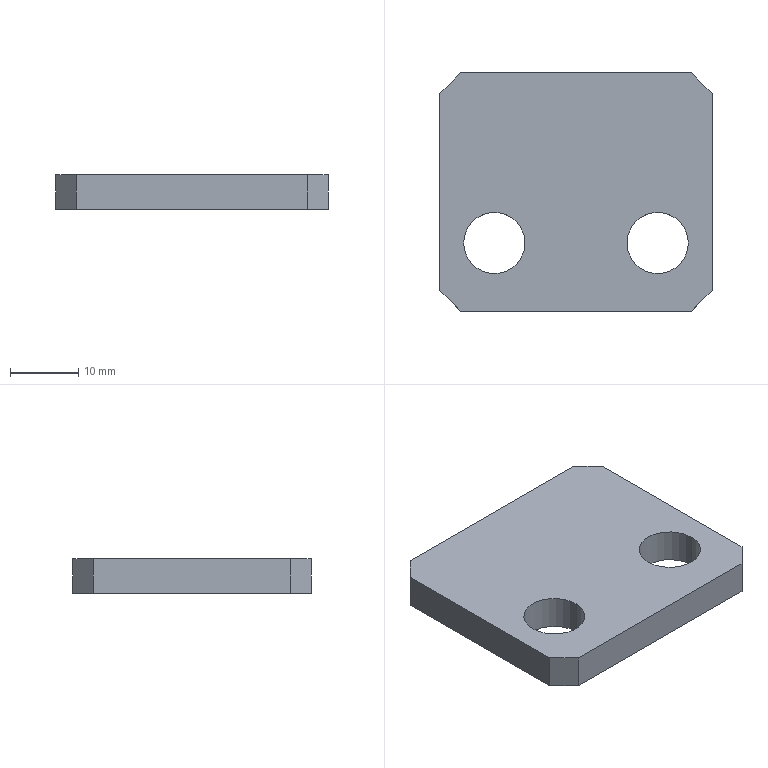Part | SolidWorks | features BaseBody 1 | 1 solid | 14 faces | box 40 x 35 x 5 mm | volume 6274 mm3 | plane 10 | cylinder 4 | commonest cylinder face diameters 9 x4
STEP:
#1=CARTESIAN_POINT('',(-16.5,-7.5,0.));
#2=VERTEX_POINT('',#1);
#3=CARTESIAN_POINT('',(-7.5,-7.5,0.));
#4=VERTEX_POINT('',#3);
#5=CARTESIAN_POINT('',(-12.,-7.5,0.));
#6=DIRECTION('',(0.,0.,1.));
#7=DIRECTION('',(1.,0.,0.));
#8=AXIS2_PLACEMENT_3D('',#5,#6,#7);
#9=CIRCLE('',#8,4.5);
#10=EDGE_CURVE('',#2,#4,#9,.T.);
#11=ORIENTED_EDGE('',*,*,#10,.F.);
#12=CARTESIAN_POINT('',(-16.5,-7.5,5.));
#13=VERTEX_POINT('',#12);
#14=CARTESIAN_POINT('',(-16.5,-7.5,5.));
#15=DIRECTION('',(0.,0.,1.));
#16=VECTOR('',#15,1000.);
#17=LINE('',#14,#16);
#18=EDGE_CURVE('',#2,#13,#17,.T.);
#19=ORIENTED_EDGE('',*,*,#18,.T.);
#20=CARTESIAN_POINT('',(-7.5,-7.5,5.));
#21=VERTEX_POINT('',#20);
#22=CARTESIAN_POINT('',(-12.,-7.5,5.));
#23=DIRECTION('',(0.,0.,1.));
#24=DIRECTION('',(1.,0.,0.));
#25=AXIS2_PLACEMENT_3D('',#22,#23,#24);
#26=CIRCLE('',#25,4.5);
#27=EDGE_CURVE('',#13,#21,#26,.T.);
#28=ORIENTED_EDGE('',*,*,#27,.T.);
#29=CARTESIAN_POINT('',(-7.5,-7.5,5.));
#30=DIRECTION('',(0.,0.,1.));
#31=VECTOR('',#30,1000.);
#32=LINE('',#29,#31);
#33=EDGE_CURVE('',#4,#21,#32,.T.);
#34=ORIENTED_EDGE('',*,*,#33,.F.);
#35=EDGE_LOOP('',(#11,#19,#28,#34));
#36=FACE_OUTER_BOUND('',#35,.T.);
#37=CARTESIAN_POINT('',(-12.,-7.5,5.));
#38=DIRECTION('',(0.,0.,1.));
#39=DIRECTION('',(1.,0.,0.));
#40=AXIS2_PLACEMENT_3D('',#37,#38,#39);
#41=CYLINDRICAL_SURFACE('',#40,4.5);
#42=ADVANCED_FACE('',(#36),#41,.F.);
#43=CARTESIAN_POINT('',(7.5,-7.5,0.));
#44=VERTEX_POINT('',#43);
#45=CARTESIAN_POINT('',(16.5,-7.5,0.));
#46=VERTEX_POINT('',#45);
#47=CARTESIAN_POINT('',(12.,-7.5,0.));
#48=DIRECTION('',(0.,0.,1.));
#49=DIRECTION('',(1.,0.,0.));
#50=AXIS2_PLACEMENT_3D('',#47,#48,#49);
#51=CIRCLE('',#50,4.5);
#52=EDGE_CURVE('',#44,#46,#51,.T.);
#53=ORIENTED_EDGE('',*,*,#52,.F.);
#54=CARTESIAN_POINT('',(7.5,-7.5,5.));
#55=VERTEX_POINT('',#54);
#56=CARTESIAN_POINT('',(7.5,-7.5,5.));
#57=DIRECTION('',(0.,0.,1.));
#58=VECTOR('',#57,1000.);
#59=LINE('',#56,#58);
#60=EDGE_CURVE('',#44,#55,#59,.T.);
#61=ORIENTED_EDGE('',*,*,#60,.T.);
#62=CARTESIAN_POINT('',(16.5,-7.5,5.));
#63=VERTEX_POINT('',#62);
#64=CARTESIAN_POINT('',(12.,-7.5,5.));
#65=DIRECTION('',(0.,0.,1.));
#66=DIRECTION('',(1.,0.,0.));
#67=AXIS2_PLACEMENT_3D('',#64,#65,#66);
#68=CIRCLE('',#67,4.5);
#69=EDGE_CURVE('',#55,#63,#68,.T.);
#70=ORIENTED_EDGE('',*,*,#69,.T.);
#71=CARTESIAN_POINT('',(16.5,-7.5,5.));
#72=DIRECTION('',(0.,0.,1.));
#73=VECTOR('',#72,1000.);
#74=LINE('',#71,#73);
#75=EDGE_CURVE('',#46,#63,#74,.T.);
#76=ORIENTED_EDGE('',*,*,#75,.F.);
#77=EDGE_LOOP('',(#53,#61,#70,#76));
#78=FACE_OUTER_BOUND('',#77,.T.);
#79=CARTESIAN_POINT('',(12.,-7.5,5.));
#80=DIRECTION('',(0.,0.,1.));
#81=DIRECTION('',(1.,0.,0.));
#82=AXIS2_PLACEMENT_3D('',#79,#80,#81);
#83=CYLINDRICAL_SURFACE('',#82,4.5);
#84=ADVANCED_FACE('',(#78),#83,.F.);
#85=CARTESIAN_POINT('',(-20.,14.5,0.));
#86=VERTEX_POINT('',#85);
#87=CARTESIAN_POINT('',(-20.,-14.5,0.));
#88=VERTEX_POINT('',#87);
#89=CARTESIAN_POINT('',(-20.,17.5,0.));
#90=DIRECTION('',(0.,-1.,0.));
#91=VECTOR('',#90,1000.);
#92=LINE('',#89,#91);
#93=EDGE_CURVE('',#86,#88,#92,.T.);
#94=ORIENTED_EDGE('',*,*,#93,.T.);
#95=CARTESIAN_POINT('',(-20.,-14.5,5.));
#96=VERTEX_POINT('',#95);
#97=CARTESIAN_POINT('',(-20.,-14.5,5.));
#98=DIRECTION('',(0.,0.,1.));
#99=VECTOR('',#98,1000.);
#100=LINE('',#97,#99);
#101=EDGE_CURVE('',#88,#96,#100,.T.);
#102=ORIENTED_EDGE('',*,*,#101,.T.);
#103=CARTESIAN_POINT('',(-20.,14.5,5.));
#104=VERTEX_POINT('',#103);
#105=CARTESIAN_POINT('',(-20.,17.5,5.));
#106=DIRECTION('',(0.,-1.,0.));
#107=VECTOR('',#106,1000.);
#108=LINE('',#105,#107);
#109=EDGE_CURVE('',#104,#96,#108,.T.);
#110=ORIENTED_EDGE('',*,*,#109,.F.);
#111=CARTESIAN_POINT('',(-20.,14.5,5.));
#112=DIRECTION('',(0.,0.,-1.));
#113=VECTOR('',#112,1000.);
#114=LINE('',#111,#113);
#115=EDGE_CURVE('',#104,#86,#114,.T.);
#116=ORIENTED_EDGE('',*,*,#115,.T.);
#117=EDGE_LOOP('',(#94,#102,#110,#116));
#118=FACE_OUTER_BOUND('',#117,.T.);
#119=CARTESIAN_POINT('',(-20.,17.5,5.));
#120=DIRECTION('',(1.,0.,0.));
#121=DIRECTION('',(0.,0.,-1.));
#122=AXIS2_PLACEMENT_3D('',#119,#120,#121);
#123=PLANE('',#122);
#124=ADVANCED_FACE('',(#118),#123,.F.);
#125=CARTESIAN_POINT('',(-17.,-17.5,5.));
#126=VERTEX_POINT('',#125);
#127=CARTESIAN_POINT('',(17.,-17.5,5.));
#128=VERTEX_POINT('',#127);
#129=CARTESIAN_POINT('',(20.,-17.5,5.));
#130=DIRECTION('',(1.,0.,0.));
#131=VECTOR('',#130,1000.);
#132=LINE('',#129,#131);
#133=EDGE_CURVE('',#126,#128,#132,.T.);
#134=ORIENTED_EDGE('',*,*,#133,.F.);
#135=CARTESIAN_POINT('',(-17.,-17.5,0.));
#136=VERTEX_POINT('',#135);
#137=CARTESIAN_POINT('',(-17.,-17.5,5.));
#138=DIRECTION('',(0.,0.,-1.));
#139=VECTOR('',#138,1000.);
#140=LINE('',#137,#139);
#141=EDGE_CURVE('',#126,#136,#140,.T.);
#142=ORIENTED_EDGE('',*,*,#141,.T.);
#143=CARTESIAN_POINT('',(17.,-17.5,0.));
#144=VERTEX_POINT('',#143);
#145=CARTESIAN_POINT('',(20.,-17.5,0.));
#146=DIRECTION('',(1.,0.,0.));
#147=VECTOR('',#146,1000.);
#148=LINE('',#145,#147);
#149=EDGE_CURVE('',#136,#144,#148,.T.);
#150=ORIENTED_EDGE('',*,*,#149,.T.);
#151=CARTESIAN_POINT('',(17.,-17.5,5.));
#152=DIRECTION('',(0.,0.,1.));
#153=VECTOR('',#152,1000.);
#154=LINE('',#151,#153);
#155=EDGE_CURVE('',#144,#128,#154,.T.);
#156=ORIENTED_EDGE('',*,*,#155,.T.);
#157=EDGE_LOOP('',(#134,#142,#150,#156));
#158=FACE_OUTER_BOUND('',#157,.T.);
#159=CARTESIAN_POINT('',(20.,-17.5,5.));
#160=DIRECTION('',(0.,1.,0.));
#161=DIRECTION('',(-1.,0.,0.));
#162=AXIS2_PLACEMENT_3D('',#159,#160,#161);
#163=PLANE('',#162);
#164=ADVANCED_FACE('',(#158),#163,.F.);
#165=CARTESIAN_POINT('',(20.,-14.5,5.));
#166=VERTEX_POINT('',#165);
#167=CARTESIAN_POINT('',(20.,14.5,5.));
#168=VERTEX_POINT('',#167);
#169=CARTESIAN_POINT('',(20.,17.5,5.));
#170=DIRECTION('',(0.,1.,0.));
#171=VECTOR('',#170,1000.);
#172=LINE('',#169,#171);
#173=EDGE_CURVE('',#166,#168,#172,.T.);
#174=ORIENTED_EDGE('',*,*,#173,.F.);
#175=CARTESIAN_POINT('',(20.,-14.5,0.));
#176=VERTEX_POINT('',#175);
#177=CARTESIAN_POINT('',(20.,-14.5,5.));
#178=DIRECTION('',(0.,0.,-1.));
#179=VECTOR('',#178,1000.);
#180=LINE('',#177,#179);
#181=EDGE_CURVE('',#166,#176,#180,.T.);
#182=ORIENTED_EDGE('',*,*,#181,.T.);
#183=CARTESIAN_POINT('',(20.,14.5,0.));
#184=VERTEX_POINT('',#183);
#185=CARTESIAN_POINT('',(20.,17.5,0.));
#186=DIRECTION('',(0.,1.,0.));
#187=VECTOR('',#186,1000.);
#188=LINE('',#185,#187);
#189=EDGE_CURVE('',#176,#184,#188,.T.);
#190=ORIENTED_EDGE('',*,*,#189,.T.);
#191=CARTESIAN_POINT('',(20.,14.5,5.));
#192=DIRECTION('',(0.,0.,1.));
#193=VECTOR('',#192,1000.);
#194=LINE('',#191,#193);
#195=EDGE_CURVE('',#184,#168,#194,.T.);
#196=ORIENTED_EDGE('',*,*,#195,.T.);
#197=EDGE_LOOP('',(#174,#182,#190,#196));
#198=FACE_OUTER_BOUND('',#197,.T.);
#199=CARTESIAN_POINT('',(20.,17.5,5.));
#200=DIRECTION('',(-1.,0.,0.));
#201=DIRECTION('',(0.,-1.,0.));
#202=AXIS2_PLACEMENT_3D('',#199,#200,#201);
#203=PLANE('',#202);
#204=ADVANCED_FACE('',(#198),#203,.F.);
#205=CARTESIAN_POINT('',(17.,17.5,5.));
#206=VERTEX_POINT('',#205);
#207=CARTESIAN_POINT('',(-17.,17.5,5.));
#208=VERTEX_POINT('',#207);
#209=CARTESIAN_POINT('',(20.,17.5,5.));
#210=DIRECTION('',(-1.,0.,0.));
#211=VECTOR('',#210,1000.);
#212=LINE('',#209,#211);
#213=EDGE_CURVE('',#206,#208,#212,.T.);
#214=ORIENTED_EDGE('',*,*,#213,.F.);
#215=CARTESIAN_POINT('',(17.,17.5,0.));
#216=VERTEX_POINT('',#215);
#217=CARTESIAN_POINT('',(17.,17.5,5.));
#218=DIRECTION('',(0.,0.,-1.));
#219=VECTOR('',#218,1000.);
#220=LINE('',#217,#219);
#221=EDGE_CURVE('',#206,#216,#220,.T.);
#222=ORIENTED_EDGE('',*,*,#221,.T.);
#223=CARTESIAN_POINT('',(-17.,17.5,0.));
#224=VERTEX_POINT('',#223);
#225=CARTESIAN_POINT('',(20.,17.5,0.));
#226=DIRECTION('',(-1.,0.,0.));
#227=VECTOR('',#226,1000.);
#228=LINE('',#225,#227);
#229=EDGE_CURVE('',#216,#224,#228,.T.);
#230=ORIENTED_EDGE('',*,*,#229,.T.);
#231=CARTESIAN_POINT('',(-17.,17.5,5.));
#232=DIRECTION('',(0.,0.,1.));
#233=VECTOR('',#232,1000.);
#234=LINE('',#231,#233);
#235=EDGE_CURVE('',#224,#208,#234,.T.);
#236=ORIENTED_EDGE('',*,*,#235,.T.);
#237=EDGE_LOOP('',(#214,#222,#230,#236));
#238=FACE_OUTER_BOUND('',#237,.T.);
#239=CARTESIAN_POINT('',(20.,17.5,5.));
#240=DIRECTION('',(0.,-1.,0.));
#241=DIRECTION('',(1.,0.,0.));
#242=AXIS2_PLACEMENT_3D('',#239,#240,#241);
#243=PLANE('',#242);
#244=ADVANCED_FACE('',(#238),#243,.F.);
#245=CARTESIAN_POINT('',(-12.,-7.5,5.));
#246=DIRECTION('',(0.,0.,1.));
#247=DIRECTION('',(1.,0.,0.));
#248=AXIS2_PLACEMENT_3D('',#245,#246,#247);
#249=CIRCLE('',#248,4.5);
#250=EDGE_CURVE('',#21,#13,#249,.T.);
#251=ORIENTED_EDGE('',*,*,#250,.F.);
#252=ORIENTED_EDGE('',*,*,#27,.F.);
#253=EDGE_LOOP('',(#251,#252));
#254=FACE_BOUND('',#253,.T.);
#255=CARTESIAN_POINT('',(12.,-7.5,5.));
#256=DIRECTION('',(0.,0.,1.));
#257=DIRECTION('',(1.,0.,0.));
#258=AXIS2_PLACEMENT_3D('',#255,#256,#257);
#259=CIRCLE('',#258,4.5);
#260=EDGE_CURVE('',#63,#55,#259,.T.);
#261=ORIENTED_EDGE('',*,*,#260,.F.);
#262=ORIENTED_EDGE('',*,*,#69,.F.);
#263=EDGE_LOOP('',(#261,#262));
#264=FACE_BOUND('',#263,.T.);
#265=ORIENTED_EDGE('',*,*,#109,.T.);
#266=CARTESIAN_POINT('',(-17.,-17.5,5.));
#267=DIRECTION('',(0.7071,-0.7071,0.));
#268=VECTOR('',#267,1000.);
#269=LINE('',#266,#268);
#270=EDGE_CURVE('',#96,#126,#269,.T.);
#271=ORIENTED_EDGE('',*,*,#270,.T.);
#272=ORIENTED_EDGE('',*,*,#133,.T.);
#273=CARTESIAN_POINT('',(20.,-14.5,5.));
#274=DIRECTION('',(0.7071,0.7071,0.));
#275=VECTOR('',#274,1000.);
#276=LINE('',#273,#275);
#277=EDGE_CURVE('',#128,#166,#276,.T.);
#278=ORIENTED_EDGE('',*,*,#277,.T.);
#279=ORIENTED_EDGE('',*,*,#173,.T.);
#280=CARTESIAN_POINT('',(17.,17.5,5.));
#281=DIRECTION('',(-0.7071,0.7071,0.));
#282=VECTOR('',#281,1000.);
#283=LINE('',#280,#282);
#284=EDGE_CURVE('',#168,#206,#283,.T.);
#285=ORIENTED_EDGE('',*,*,#284,.T.);
#286=ORIENTED_EDGE('',*,*,#213,.T.);
#287=CARTESIAN_POINT('',(-20.,14.5,5.));
#288=DIRECTION('',(-0.7071,-0.7071,0.));
#289=VECTOR('',#288,1000.);
#290=LINE('',#287,#289);
#291=EDGE_CURVE('',#208,#104,#290,.T.);
#292=ORIENTED_EDGE('',*,*,#291,.T.);
#293=EDGE_LOOP('',(#265,#271,#272,#278,#279,#285,#286,#292));
#294=FACE_OUTER_BOUND('',#293,.T.);
#295=CARTESIAN_POINT('',(0.,0.,5.));
#296=DIRECTION('',(0.,0.,-1.));
#297=DIRECTION('',(-1.,0.,0.));
#298=AXIS2_PLACEMENT_3D('',#295,#296,#297);
#299=PLANE('',#298);
#300=ADVANCED_FACE('',(#254,#264,#294),#299,.F.);
#301=CARTESIAN_POINT('',(-12.,-7.5,0.));
#302=DIRECTION('',(0.,0.,1.));
#303=DIRECTION('',(1.,0.,0.));
#304=AXIS2_PLACEMENT_3D('',#301,#302,#303);
#305=CIRCLE('',#304,4.5);
#306=EDGE_CURVE('',#4,#2,#305,.T.);
#307=ORIENTED_EDGE('',*,*,#306,.T.);
#308=ORIENTED_EDGE('',*,*,#10,.T.);
#309=EDGE_LOOP('',(#307,#308));
#310=FACE_BOUND('',#309,.T.);
#311=CARTESIAN_POINT('',(12.,-7.5,0.));
#312=DIRECTION('',(0.,0.,1.));
#313=DIRECTION('',(1.,0.,0.));
#314=AXIS2_PLACEMENT_3D('',#311,#312,#313);
#315=CIRCLE('',#314,4.5);
#316=EDGE_CURVE('',#46,#44,#315,.T.);
#317=ORIENTED_EDGE('',*,*,#316,.T.);
#318=ORIENTED_EDGE('',*,*,#52,.T.);
#319=EDGE_LOOP('',(#317,#318));
#320=FACE_BOUND('',#319,.T.);
#321=ORIENTED_EDGE('',*,*,#149,.F.);
#322=CARTESIAN_POINT('',(-17.25,-17.25,0.));
#323=DIRECTION('',(-0.7071,0.7071,0.));
#324=VECTOR('',#323,1000.);
#325=LINE('',#322,#324);
#326=EDGE_CURVE('',#136,#88,#325,.T.);
#327=ORIENTED_EDGE('',*,*,#326,.T.);
#328=ORIENTED_EDGE('',*,*,#93,.F.);
#329=CARTESIAN_POINT('',(-17.25,17.25,0.));
#330=DIRECTION('',(0.7071,0.7071,0.));
#331=VECTOR('',#330,1000.);
#332=LINE('',#329,#331);
#333=EDGE_CURVE('',#86,#224,#332,.T.);
#334=ORIENTED_EDGE('',*,*,#333,.T.);
#335=ORIENTED_EDGE('',*,*,#229,.F.);
#336=CARTESIAN_POINT('',(17.25,17.25,0.));
#337=DIRECTION('',(0.7071,-0.7071,0.));
#338=VECTOR('',#337,1000.);
#339=LINE('',#336,#338);
#340=EDGE_CURVE('',#216,#184,#339,.T.);
#341=ORIENTED_EDGE('',*,*,#340,.T.);
#342=ORIENTED_EDGE('',*,*,#189,.F.);
#343=CARTESIAN_POINT('',(17.25,-17.25,0.));
#344=DIRECTION('',(-0.7071,-0.7071,0.));
#345=VECTOR('',#344,1000.);
#346=LINE('',#343,#345);
#347=EDGE_CURVE('',#176,#144,#346,.T.);
#348=ORIENTED_EDGE('',*,*,#347,.T.);
#349=EDGE_LOOP('',(#321,#327,#328,#334,#335,#341,#342,#348));
#350=FACE_OUTER_BOUND('',#349,.T.);
#351=CARTESIAN_POINT('',(0.,0.,0.));
#352=DIRECTION('',(0.,0.,-1.));
#353=DIRECTION('',(-1.,0.,0.));
#354=AXIS2_PLACEMENT_3D('',#351,#352,#353);
#355=PLANE('',#354);
#356=ADVANCED_FACE('',(#310,#320,#350),#355,.T.);
#357=ORIENTED_EDGE('',*,*,#270,.F.);
#358=ORIENTED_EDGE('',*,*,#101,.F.);
#359=ORIENTED_EDGE('',*,*,#326,.F.);
#360=ORIENTED_EDGE('',*,*,#141,.F.);
#361=EDGE_LOOP('',(#357,#358,#359,#360));
#362=FACE_OUTER_BOUND('',#361,.T.);
#363=CARTESIAN_POINT('',(-17.,-17.5,5.));
#364=DIRECTION('',(0.7071,0.7071,0.));
#365=DIRECTION('',(0.,0.,-1.));
#366=AXIS2_PLACEMENT_3D('',#363,#364,#365);
#367=PLANE('',#366);
#368=ADVANCED_FACE('',(#362),#367,.F.);
#369=ORIENTED_EDGE('',*,*,#277,.F.);
#370=ORIENTED_EDGE('',*,*,#155,.F.);
#371=ORIENTED_EDGE('',*,*,#347,.F.);
#372=ORIENTED_EDGE('',*,*,#181,.F.);
#373=EDGE_LOOP('',(#369,#370,#371,#372));
#374=FACE_OUTER_BOUND('',#373,.T.);
#375=CARTESIAN_POINT('',(20.,-14.5,5.));
#376=DIRECTION('',(-0.7071,0.7071,0.));
#377=DIRECTION('',(0.,0.,-1.));
#378=AXIS2_PLACEMENT_3D('',#375,#376,#377);
#379=PLANE('',#378);
#380=ADVANCED_FACE('',(#374),#379,.F.);
#381=ORIENTED_EDGE('',*,*,#284,.F.);
#382=ORIENTED_EDGE('',*,*,#195,.F.);
#383=ORIENTED_EDGE('',*,*,#340,.F.);
#384=ORIENTED_EDGE('',*,*,#221,.F.);
#385=EDGE_LOOP('',(#381,#382,#383,#384));
#386=FACE_OUTER_BOUND('',#385,.T.);
#387=CARTESIAN_POINT('',(17.,17.5,5.));
#388=DIRECTION('',(-0.7071,-0.7071,0.));
#389=DIRECTION('',(0.,0.,-1.));
#390=AXIS2_PLACEMENT_3D('',#387,#388,#389);
#391=PLANE('',#390);
#392=ADVANCED_FACE('',(#386),#391,.F.);
#393=ORIENTED_EDGE('',*,*,#291,.F.);
#394=ORIENTED_EDGE('',*,*,#235,.F.);
#395=ORIENTED_EDGE('',*,*,#333,.F.);
#396=ORIENTED_EDGE('',*,*,#115,.F.);
#397=EDGE_LOOP('',(#393,#394,#395,#396));
#398=FACE_OUTER_BOUND('',#397,.T.);
#399=CARTESIAN_POINT('',(-20.,14.5,5.));
#400=DIRECTION('',(0.7071,-0.7071,0.));
#401=DIRECTION('',(0.,0.,-1.));
#402=AXIS2_PLACEMENT_3D('',#399,#400,#401);
#403=PLANE('',#402);
#404=ADVANCED_FACE('',(#398),#403,.F.);
#405=ORIENTED_EDGE('',*,*,#60,.F.);
#406=ORIENTED_EDGE('',*,*,#316,.F.);
#407=ORIENTED_EDGE('',*,*,#75,.T.);
#408=ORIENTED_EDGE('',*,*,#260,.T.);
#409=EDGE_LOOP('',(#405,#406,#407,#408));
#410=FACE_OUTER_BOUND('',#409,.T.);
#411=CARTESIAN_POINT('',(12.,-7.5,5.));
#412=DIRECTION('',(0.,0.,1.));
#413=DIRECTION('',(1.,0.,0.));
#414=AXIS2_PLACEMENT_3D('',#411,#412,#413);
#415=CYLINDRICAL_SURFACE('',#414,4.5);
#416=ADVANCED_FACE('',(#410),#415,.F.);
#417=ORIENTED_EDGE('',*,*,#18,.F.);
#418=ORIENTED_EDGE('',*,*,#306,.F.);
#419=ORIENTED_EDGE('',*,*,#33,.T.);
#420=ORIENTED_EDGE('',*,*,#250,.T.);
#421=EDGE_LOOP('',(#417,#418,#419,#420));
#422=FACE_OUTER_BOUND('',#421,.T.);
#423=CARTESIAN_POINT('',(-12.,-7.5,5.));
#424=DIRECTION('',(0.,0.,1.));
#425=DIRECTION('',(1.,0.,0.));
#426=AXIS2_PLACEMENT_3D('',#423,#424,#425);
#427=CYLINDRICAL_SURFACE('',#426,4.5);
#428=ADVANCED_FACE('',(#422),#427,.F.);
#429=CLOSED_SHELL('',(#42,#84,#124,#164,#204,#244,#300,#356,#368,#380,#392,#404,#416,#428));
#430=MANIFOLD_SOLID_BREP('',#429);
#431=CARTESIAN_POINT('',(0.,0.,0.));
#432=DIRECTION('',(0.,0.,1.));
#433=DIRECTION('',(1.,0.,0.));
#434=AXIS2_PLACEMENT_3D('',#431,#432,#433);
#435=(LENGTH_UNIT()NAMED_UNIT(*)SI_UNIT(.MILLI.,.METRE.));
#436=UNCERTAINTY_MEASURE_WITH_UNIT(LENGTH_MEASURE(0.00001),#435,'','');
#437=(NAMED_UNIT(*)PLANE_ANGLE_UNIT()SI_UNIT($,.RADIAN.));
#438=(NAMED_UNIT(*)SI_UNIT($,.STERADIAN.)SOLID_ANGLE_UNIT());
#439=(GEOMETRIC_REPRESENTATION_CONTEXT(3)GLOBAL_UNCERTAINTY_ASSIGNED_CONTEXT((#436))GLOBAL_UNIT_ASSIGNED_CONTEXT((#435,#437,#438))REPRESENTATION_CONTEXT('',''));
#440=ADVANCED_BREP_SHAPE_REPRESENTATION('',(#430,#434),#439);